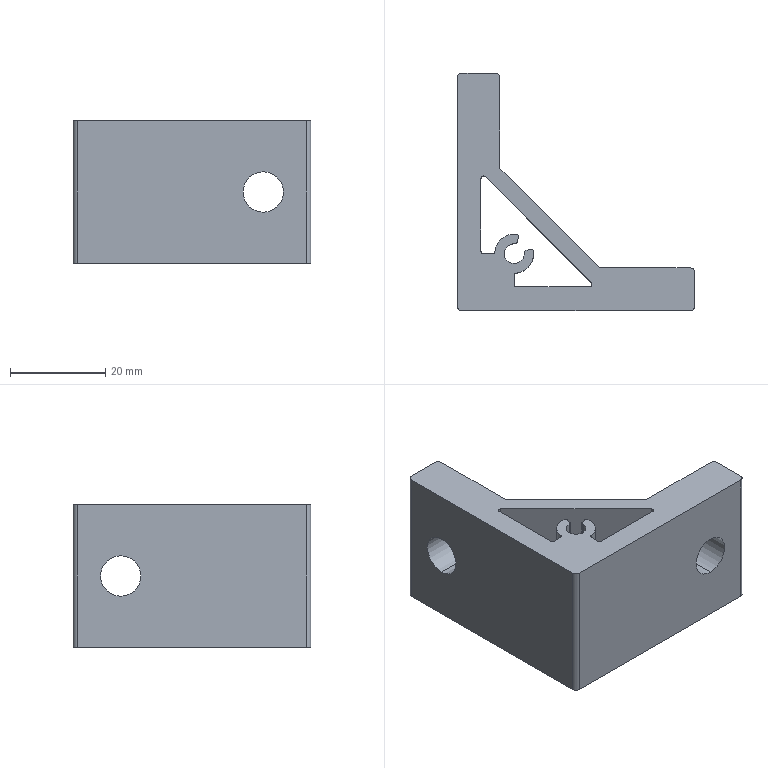Part | SolidWorks | features BaseBody 1 | 1 solid | 41 faces | box 50 x 50 x 30 mm | volume 23521 mm3 | cylinder 25 | plane 16 | commonest cylinder face diameters 1 x11 2 x5 8.5 x4 4.2 x3 8.2 x2
STEP:
#1=CARTESIAN_POINT('',(0.,40.,-10.75));
#2=VERTEX_POINT('',#1);
#3=CARTESIAN_POINT('',(0.,40.,-19.25));
#4=VERTEX_POINT('',#3);
#5=CARTESIAN_POINT('',(0.,40.,-15.));
#6=DIRECTION('',(1.,0.,0.));
#7=DIRECTION('',(0.,0.,-1.));
#8=AXIS2_PLACEMENT_3D('',#5,#6,#7);
#9=CIRCLE('',#8,4.25);
#10=EDGE_CURVE('',#2,#4,#9,.T.);
#11=ORIENTED_EDGE('',*,*,#10,.F.);
#12=CARTESIAN_POINT('',(9.,40.,-10.75));
#13=VERTEX_POINT('',#12);
#14=CARTESIAN_POINT('',(30.,40.,-10.75));
#15=DIRECTION('',(1.,0.,0.));
#16=VECTOR('',#15,1000.);
#17=LINE('',#14,#16);
#18=EDGE_CURVE('',#2,#13,#17,.T.);
#19=ORIENTED_EDGE('',*,*,#18,.T.);
#20=CARTESIAN_POINT('',(9.,40.,-19.25));
#21=VERTEX_POINT('',#20);
#22=CARTESIAN_POINT('',(9.,40.,-15.));
#23=DIRECTION('',(-1.,0.,0.));
#24=DIRECTION('',(0.,0.,-1.));
#25=AXIS2_PLACEMENT_3D('',#22,#23,#24);
#26=CIRCLE('',#25,4.25);
#27=EDGE_CURVE('',#21,#13,#26,.T.);
#28=ORIENTED_EDGE('',*,*,#27,.F.);
#29=CARTESIAN_POINT('',(30.,40.,-19.25));
#30=DIRECTION('',(1.,0.,0.));
#31=VECTOR('',#30,1000.);
#32=LINE('',#29,#31);
#33=EDGE_CURVE('',#4,#21,#32,.T.);
#34=ORIENTED_EDGE('',*,*,#33,.F.);
#35=EDGE_LOOP('',(#11,#19,#28,#34));
#36=FACE_OUTER_BOUND('',#35,.T.);
#37=CARTESIAN_POINT('',(30.,40.,-15.));
#38=DIRECTION('',(1.,0.,0.));
#39=DIRECTION('',(0.,0.,-1.));
#40=AXIS2_PLACEMENT_3D('',#37,#38,#39);
#41=CYLINDRICAL_SURFACE('',#40,4.25);
#42=ADVANCED_FACE('',(#36),#41,.F.);
#43=CARTESIAN_POINT('',(14.1,12.,0.));
#44=VERTEX_POINT('',#43);
#45=CARTESIAN_POINT('',(9.9,12.,0.));
#46=VERTEX_POINT('',#45);
#47=CARTESIAN_POINT('',(12.,12.,0.));
#48=DIRECTION('',(0.,0.,-1.));
#49=DIRECTION('',(-1.,0.,0.));
#50=AXIS2_PLACEMENT_3D('',#47,#48,#49);
#51=CIRCLE('',#50,2.1);
#52=EDGE_CURVE('',#44,#46,#51,.T.);
#53=ORIENTED_EDGE('',*,*,#52,.F.);
#54=CARTESIAN_POINT('',(14.1,12.,-30.));
#55=VERTEX_POINT('',#54);
#56=CARTESIAN_POINT('',(14.1,12.,-30.));
#57=DIRECTION('',(0.,0.,-1.));
#58=VECTOR('',#57,1000.);
#59=LINE('',#56,#58);
#60=EDGE_CURVE('',#44,#55,#59,.T.);
#61=ORIENTED_EDGE('',*,*,#60,.T.);
#62=CARTESIAN_POINT('',(9.9,12.,-30.));
#63=VERTEX_POINT('',#62);
#64=CARTESIAN_POINT('',(12.,12.,-30.));
#65=DIRECTION('',(0.,0.,-1.));
#66=DIRECTION('',(-1.,0.,0.));
#67=AXIS2_PLACEMENT_3D('',#64,#65,#66);
#68=CIRCLE('',#67,2.1);
#69=EDGE_CURVE('',#55,#63,#68,.T.);
#70=ORIENTED_EDGE('',*,*,#69,.T.);
#71=CARTESIAN_POINT('',(9.9,12.,-30.));
#72=DIRECTION('',(0.,0.,-1.));
#73=VECTOR('',#72,1000.);
#74=LINE('',#71,#73);
#75=EDGE_CURVE('',#46,#63,#74,.T.);
#76=ORIENTED_EDGE('',*,*,#75,.F.);
#77=EDGE_LOOP('',(#53,#61,#70,#76));
#78=FACE_OUTER_BOUND('',#77,.T.);
#79=CARTESIAN_POINT('',(12.,12.,-30.));
#80=DIRECTION('',(0.,0.,-1.));
#81=DIRECTION('',(-1.,0.,0.));
#82=AXIS2_PLACEMENT_3D('',#79,#80,#81);
#83=CYLINDRICAL_SURFACE('',#82,2.1);
#84=ADVANCED_FACE('',(#78),#83,.F.);
#85=CARTESIAN_POINT('',(12.143,14.095,0.));
#86=VERTEX_POINT('',#85);
#87=CARTESIAN_POINT('',(12.,12.,0.));
#88=DIRECTION('',(0.,0.,-1.));
#89=DIRECTION('',(-1.,0.,0.));
#90=AXIS2_PLACEMENT_3D('',#87,#88,#89);
#91=CIRCLE('',#90,2.1);
#92=EDGE_CURVE('',#46,#86,#91,.T.);
#93=ORIENTED_EDGE('',*,*,#92,.F.);
#94=ORIENTED_EDGE('',*,*,#75,.T.);
#95=CARTESIAN_POINT('',(12.143,14.095,-30.));
#96=VERTEX_POINT('',#95);
#97=CARTESIAN_POINT('',(12.,12.,-30.));
#98=DIRECTION('',(0.,0.,-1.));
#99=DIRECTION('',(-1.,0.,0.));
#100=AXIS2_PLACEMENT_3D('',#97,#98,#99);
#101=CIRCLE('',#100,2.1);
#102=EDGE_CURVE('',#63,#96,#101,.T.);
#103=ORIENTED_EDGE('',*,*,#102,.T.);
#104=CARTESIAN_POINT('',(12.143,14.095,-30.));
#105=DIRECTION('',(0.,0.,-1.));
#106=VECTOR('',#105,1000.);
#107=LINE('',#104,#106);
#108=EDGE_CURVE('',#86,#96,#107,.T.);
#109=ORIENTED_EDGE('',*,*,#108,.F.);
#110=EDGE_LOOP('',(#93,#94,#103,#109));
#111=FACE_OUTER_BOUND('',#110,.T.);
#112=CARTESIAN_POINT('',(12.,12.,-30.));
#113=DIRECTION('',(0.,0.,-1.));
#114=DIRECTION('',(-1.,0.,0.));
#115=AXIS2_PLACEMENT_3D('',#112,#113,#114);
#116=CYLINDRICAL_SURFACE('',#115,2.1);
#117=ADVANCED_FACE('',(#111),#116,.F.);
#118=CARTESIAN_POINT('',(40.,0.,-19.25));
#119=VERTEX_POINT('',#118);
#120=CARTESIAN_POINT('',(40.,0.,-10.75));
#121=VERTEX_POINT('',#120);
#122=CARTESIAN_POINT('',(40.,0.,-15.));
#123=DIRECTION('',(0.,1.,0.));
#124=DIRECTION('',(0.,0.,1.));
#125=AXIS2_PLACEMENT_3D('',#122,#123,#124);
#126=CIRCLE('',#125,4.25);
#127=EDGE_CURVE('',#119,#121,#126,.T.);
#128=ORIENTED_EDGE('',*,*,#127,.F.);
#129=CARTESIAN_POINT('',(40.,9.,-19.25));
#130=VERTEX_POINT('',#129);
#131=CARTESIAN_POINT('',(40.,30.,-19.25));
#132=DIRECTION('',(0.,1.,0.));
#133=VECTOR('',#132,1000.);
#134=LINE('',#131,#133);
#135=EDGE_CURVE('',#119,#130,#134,.T.);
#136=ORIENTED_EDGE('',*,*,#135,.T.);
#137=CARTESIAN_POINT('',(40.,9.,-10.75));
#138=VERTEX_POINT('',#137);
#139=CARTESIAN_POINT('',(40.,9.,-15.));
#140=DIRECTION('',(0.,-1.,0.));
#141=DIRECTION('',(0.,0.,1.));
#142=AXIS2_PLACEMENT_3D('',#139,#140,#141);
#143=CIRCLE('',#142,4.25);
#144=EDGE_CURVE('',#138,#130,#143,.T.);
#145=ORIENTED_EDGE('',*,*,#144,.F.);
#146=CARTESIAN_POINT('',(40.,30.,-10.75));
#147=DIRECTION('',(0.,1.,0.));
#148=VECTOR('',#147,1000.);
#149=LINE('',#146,#148);
#150=EDGE_CURVE('',#121,#138,#149,.T.);
#151=ORIENTED_EDGE('',*,*,#150,.F.);
#152=EDGE_LOOP('',(#128,#136,#145,#151));
#153=FACE_OUTER_BOUND('',#152,.T.);
#154=CARTESIAN_POINT('',(40.,30.,-15.));
#155=DIRECTION('',(0.,1.,0.));
#156=DIRECTION('',(0.,0.,1.));
#157=AXIS2_PLACEMENT_3D('',#154,#155,#156);
#158=CYLINDRICAL_SURFACE('',#157,4.25);
#159=ADVANCED_FACE('',(#153),#158,.F.);
#160=CARTESIAN_POINT('',(14.095,12.144,0.));
#161=VERTEX_POINT('',#160);
#162=CARTESIAN_POINT('',(14.094,12.178,0.));
#163=VERTEX_POINT('',#162);
#164=CARTESIAN_POINT('',(14.594,12.178,0.));
#165=DIRECTION('',(0.,0.,-1.));
#166=DIRECTION('',(-1.,0.,0.));
#167=AXIS2_PLACEMENT_3D('',#164,#165,#166);
#168=CIRCLE('',#167,0.5);
#169=EDGE_CURVE('',#161,#163,#168,.T.);
#170=ORIENTED_EDGE('',*,*,#169,.T.);
#171=CARTESIAN_POINT('',(14.094,12.178,-30.));
#172=VERTEX_POINT('',#171);
#173=CARTESIAN_POINT('',(14.094,12.178,-30.));
#174=DIRECTION('',(0.,0.,-1.));
#175=VECTOR('',#174,1000.);
#176=LINE('',#173,#175);
#177=EDGE_CURVE('',#163,#172,#176,.T.);
#178=ORIENTED_EDGE('',*,*,#177,.T.);
#179=CARTESIAN_POINT('',(14.095,12.144,-30.));
#180=VERTEX_POINT('',#179);
#181=CARTESIAN_POINT('',(14.594,12.178,-30.));
#182=DIRECTION('',(0.,0.,1.));
#183=DIRECTION('',(-1.,0.,0.));
#184=AXIS2_PLACEMENT_3D('',#181,#182,#183);
#185=CIRCLE('',#184,0.5);
#186=EDGE_CURVE('',#172,#180,#185,.T.);
#187=ORIENTED_EDGE('',*,*,#186,.T.);
#188=CARTESIAN_POINT('',(14.095,12.144,-30.));
#189=DIRECTION('',(0.,0.,1.));
#190=VECTOR('',#189,1000.);
#191=LINE('',#188,#190);
#192=EDGE_CURVE('',#180,#161,#191,.T.);
#193=ORIENTED_EDGE('',*,*,#192,.T.);
#194=EDGE_LOOP('',(#170,#178,#187,#193));
#195=FACE_OUTER_BOUND('',#194,.T.);
#196=CARTESIAN_POINT('',(14.594,12.178,-30.));
#197=DIRECTION('',(0.,0.,-1.));
#198=DIRECTION('',(-1.,0.,0.));
#199=AXIS2_PLACEMENT_3D('',#196,#197,#198);
#200=CYLINDRICAL_SURFACE('',#199,0.5);
#201=ADVANCED_FACE('',(#195),#200,.T.);
#202=CARTESIAN_POINT('',(0.,49.,-30.));
#203=VERTEX_POINT('',#202);
#204=CARTESIAN_POINT('',(0.,1.,-30.));
#205=VERTEX_POINT('',#204);
#206=CARTESIAN_POINT('',(0.,49.,-30.));
#207=DIRECTION('',(0.,-1.,0.));
#208=VECTOR('',#207,1000.);
#209=LINE('',#206,#208);
#210=EDGE_CURVE('',#203,#205,#209,.T.);
#211=ORIENTED_EDGE('',*,*,#210,.T.);
#212=CARTESIAN_POINT('',(0.,1.,0.));
#213=VERTEX_POINT('',#212);
#214=CARTESIAN_POINT('',(0.,1.,-30.));
#215=DIRECTION('',(0.,0.,1.));
#216=VECTOR('',#215,1000.);
#217=LINE('',#214,#216);
#218=EDGE_CURVE('',#205,#213,#217,.T.);
#219=ORIENTED_EDGE('',*,*,#218,.T.);
#220=CARTESIAN_POINT('',(0.,49.,0.));
#221=VERTEX_POINT('',#220);
#222=CARTESIAN_POINT('',(0.,49.,0.));
#223=DIRECTION('',(0.,1.,0.));
#224=VECTOR('',#223,1000.);
#225=LINE('',#222,#224);
#226=EDGE_CURVE('',#213,#221,#225,.T.);
#227=ORIENTED_EDGE('',*,*,#226,.T.);
#228=CARTESIAN_POINT('',(0.,49.,-30.));
#229=DIRECTION('',(0.,0.,-1.));
#230=VECTOR('',#229,1000.);
#231=LINE('',#228,#230);
#232=EDGE_CURVE('',#221,#203,#231,.T.);
#233=ORIENTED_EDGE('',*,*,#232,.T.);
#234=EDGE_LOOP('',(#211,#219,#227,#233));
#235=FACE_OUTER_BOUND('',#234,.T.);
#236=CARTESIAN_POINT('',(0.,40.,-15.));
#237=DIRECTION('',(1.,0.,0.));
#238=DIRECTION('',(0.,0.,-1.));
#239=AXIS2_PLACEMENT_3D('',#236,#237,#238);
#240=CIRCLE('',#239,4.25);
#241=EDGE_CURVE('',#4,#2,#240,.T.);
#242=ORIENTED_EDGE('',*,*,#241,.T.);
#243=ORIENTED_EDGE('',*,*,#10,.T.);
#244=EDGE_LOOP('',(#242,#243));
#245=FACE_BOUND('',#244,.T.);
#246=CARTESIAN_POINT('',(0.,49.,-30.));
#247=DIRECTION('',(-1.,0.,0.));
#248=DIRECTION('',(0.,0.,1.));
#249=AXIS2_PLACEMENT_3D('',#246,#247,#248);
#250=PLANE('',#249);
#251=ADVANCED_FACE('',(#235,#245),#250,.T.);
#252=CARTESIAN_POINT('',(1.,0.,-30.));
#253=VERTEX_POINT('',#252);
#254=CARTESIAN_POINT('',(1.,1.,-30.));
#255=DIRECTION('',(0.,0.,1.));
#256=DIRECTION('',(-1.,0.,0.));
#257=AXIS2_PLACEMENT_3D('',#254,#255,#256);
#258=CIRCLE('',#257,1.);
#259=EDGE_CURVE('',#205,#253,#258,.T.);
#260=ORIENTED_EDGE('',*,*,#259,.T.);
#261=CARTESIAN_POINT('',(1.,0.,0.));
#262=VERTEX_POINT('',#261);
#263=CARTESIAN_POINT('',(1.,0.,-30.));
#264=DIRECTION('',(0.,0.,1.));
#265=VECTOR('',#264,1000.);
#266=LINE('',#263,#265);
#267=EDGE_CURVE('',#253,#262,#266,.T.);
#268=ORIENTED_EDGE('',*,*,#267,.T.);
#269=CARTESIAN_POINT('',(1.,1.,0.));
#270=DIRECTION('',(0.,0.,-1.));
#271=DIRECTION('',(-1.,0.,0.));
#272=AXIS2_PLACEMENT_3D('',#269,#270,#271);
#273=CIRCLE('',#272,1.);
#274=EDGE_CURVE('',#262,#213,#273,.T.);
#275=ORIENTED_EDGE('',*,*,#274,.T.);
#276=ORIENTED_EDGE('',*,*,#218,.F.);
#277=EDGE_LOOP('',(#260,#268,#275,#276));
#278=FACE_OUTER_BOUND('',#277,.T.);
#279=CARTESIAN_POINT('',(1.,1.,-30.));
#280=DIRECTION('',(0.,0.,-1.));
#281=DIRECTION('',(-1.,0.,0.));
#282=AXIS2_PLACEMENT_3D('',#279,#280,#281);
#283=CYLINDRICAL_SURFACE('',#282,1.);
#284=ADVANCED_FACE('',(#278),#283,.T.);
#285=CARTESIAN_POINT('',(8.,50.,-30.));
#286=VERTEX_POINT('',#285);
#287=CARTESIAN_POINT('',(1.,50.,-30.));
#288=VERTEX_POINT('',#287);
#289=CARTESIAN_POINT('',(1.,50.,-30.));
#290=DIRECTION('',(-1.,0.,0.));
#291=VECTOR('',#290,1000.);
#292=LINE('',#289,#291);
#293=EDGE_CURVE('',#286,#288,#292,.T.);
#294=ORIENTED_EDGE('',*,*,#293,.F.);
#295=CARTESIAN_POINT('',(9.,49.,-30.));
#296=VERTEX_POINT('',#295);
#297=CARTESIAN_POINT('',(8.,49.,-30.));
#298=DIRECTION('',(0.,0.,1.));
#299=DIRECTION('',(-1.,0.,0.));
#300=AXIS2_PLACEMENT_3D('',#297,#298,#299);
#301=CIRCLE('',#300,1.);
#302=EDGE_CURVE('',#296,#286,#301,.T.);
#303=ORIENTED_EDGE('',*,*,#302,.F.);
#304=CARTESIAN_POINT('',(9.,30.,-30.));
#305=VERTEX_POINT('',#304);
#306=CARTESIAN_POINT('',(9.,49.,-30.));
#307=DIRECTION('',(0.,1.,0.));
#308=VECTOR('',#307,1000.);
#309=LINE('',#306,#308);
#310=EDGE_CURVE('',#305,#296,#309,.T.);
#311=ORIENTED_EDGE('',*,*,#310,.F.);
#312=CARTESIAN_POINT('',(30.,9.,-30.));
#313=VERTEX_POINT('',#312);
#314=CARTESIAN_POINT('',(30.,9.,-30.));
#315=DIRECTION('',(-0.7071,0.7071,0.));
#316=VECTOR('',#315,1000.);
#317=LINE('',#314,#316);
#318=EDGE_CURVE('',#313,#305,#317,.T.);
#319=ORIENTED_EDGE('',*,*,#318,.F.);
#320=CARTESIAN_POINT('',(49.,9.,-30.));
#321=VERTEX_POINT('',#320);
#322=CARTESIAN_POINT('',(1.,9.,-30.));
#323=DIRECTION('',(-1.,0.,0.));
#324=VECTOR('',#323,1000.);
#325=LINE('',#322,#324);
#326=EDGE_CURVE('',#321,#313,#325,.T.);
#327=ORIENTED_EDGE('',*,*,#326,.F.);
#328=CARTESIAN_POINT('',(50.,8.,-30.));
#329=VERTEX_POINT('',#328);
#330=CARTESIAN_POINT('',(49.,8.,-30.));
#331=DIRECTION('',(0.,0.,1.));
#332=DIRECTION('',(-1.,0.,0.));
#333=AXIS2_PLACEMENT_3D('',#330,#331,#332);
#334=CIRCLE('',#333,1.);
#335=EDGE_CURVE('',#329,#321,#334,.T.);
#336=ORIENTED_EDGE('',*,*,#335,.F.);
#337=CARTESIAN_POINT('',(50.,1.,-30.));
#338=VERTEX_POINT('',#337);
#339=CARTESIAN_POINT('',(50.,49.,-30.));
#340=DIRECTION('',(0.,1.,0.));
#341=VECTOR('',#340,1000.);
#342=LINE('',#339,#341);
#343=EDGE_CURVE('',#338,#329,#342,.T.);
#344=ORIENTED_EDGE('',*,*,#343,.F.);
#345=CARTESIAN_POINT('',(49.,0.,-30.));
#346=VERTEX_POINT('',#345);
#347=CARTESIAN_POINT('',(49.,1.,-30.));
#348=DIRECTION('',(0.,0.,1.));
#349=DIRECTION('',(-1.,0.,0.));
#350=AXIS2_PLACEMENT_3D('',#347,#348,#349);
#351=CIRCLE('',#350,1.);
#352=EDGE_CURVE('',#346,#338,#351,.T.);
#353=ORIENTED_EDGE('',*,*,#352,.F.);
#354=CARTESIAN_POINT('',(1.,0.,-30.));
#355=DIRECTION('',(1.,0.,0.));
#356=VECTOR('',#355,1000.);
#357=LINE('',#354,#356);
#358=EDGE_CURVE('',#253,#346,#357,.T.);
#359=ORIENTED_EDGE('',*,*,#358,.F.);
#360=ORIENTED_EDGE('',*,*,#259,.F.);
#361=ORIENTED_EDGE('',*,*,#210,.F.);
#362=CARTESIAN_POINT('',(1.,49.,-30.));
#363=DIRECTION('',(0.,0.,1.));
#364=DIRECTION('',(-1.,0.,0.));
#365=AXIS2_PLACEMENT_3D('',#362,#363,#364);
#366=CIRCLE('',#365,1.);
#367=EDGE_CURVE('',#288,#203,#366,.T.);
#368=ORIENTED_EDGE('',*,*,#367,.F.);
#369=EDGE_LOOP('',(#294,#303,#311,#319,#327,#336,#344,#353,#359,#360,#361,#368));
#370=FACE_OUTER_BOUND('',#369,.T.);
#371=CARTESIAN_POINT('',(5.,12.5,-30.));
#372=VERTEX_POINT('',#371);
#373=CARTESIAN_POINT('',(5.5,12.,-30.));
#374=VERTEX_POINT('',#373);
#375=CARTESIAN_POINT('',(5.5,12.5,-30.));
#376=DIRECTION('',(0.,0.,1.));
#377=DIRECTION('',(-1.,0.,0.));
#378=AXIS2_PLACEMENT_3D('',#375,#376,#377);
#379=CIRCLE('',#378,0.5);
#380=EDGE_CURVE('',#372,#374,#379,.T.);
#381=ORIENTED_EDGE('',*,*,#380,.T.);
#382=CARTESIAN_POINT('',(7.427,12.,-30.));
#383=VERTEX_POINT('',#382);
#384=CARTESIAN_POINT('',(1.,12.,-30.));
#385=DIRECTION('',(-1.,0.,0.));
#386=VECTOR('',#385,1000.);
#387=LINE('',#384,#386);
#388=EDGE_CURVE('',#383,#374,#387,.T.);
#389=ORIENTED_EDGE('',*,*,#388,.F.);
#390=CARTESIAN_POINT('',(7.924,12.446,-30.));
#391=VERTEX_POINT('',#390);
#392=CARTESIAN_POINT('',(7.427,12.5,-30.));
#393=DIRECTION('',(0.,0.,1.));
#394=DIRECTION('',(-1.,0.,0.));
#395=AXIS2_PLACEMENT_3D('',#392,#393,#394);
#396=CIRCLE('',#395,0.5);
#397=EDGE_CURVE('',#383,#391,#396,.T.);
#398=ORIENTED_EDGE('',*,*,#397,.T.);
#399=CARTESIAN_POINT('',(12.501,16.07,-30.));
#400=VERTEX_POINT('',#399);
#401=CARTESIAN_POINT('',(12.,12.001,-30.));
#402=DIRECTION('',(0.,0.,1.));
#403=DIRECTION('',(-1.,0.,0.));
#404=AXIS2_PLACEMENT_3D('',#401,#402,#403);
#405=CIRCLE('',#404,4.1);
#406=EDGE_CURVE('',#400,#391,#405,.T.);
#407=ORIENTED_EDGE('',*,*,#406,.F.);
#408=CARTESIAN_POINT('',(12.923,15.444,-30.));
#409=VERTEX_POINT('',#408);
#410=CARTESIAN_POINT('',(12.44,15.574,-30.));
#411=DIRECTION('',(0.,0.,1.));
#412=DIRECTION('',(-1.,0.,0.));
#413=AXIS2_PLACEMENT_3D('',#410,#411,#412);
#414=CIRCLE('',#413,0.5);
#415=EDGE_CURVE('',#409,#400,#414,.T.);
#416=ORIENTED_EDGE('',*,*,#415,.F.);
#417=CARTESIAN_POINT('',(12.66,14.464,-30.));
#418=VERTEX_POINT('',#417);
#419=CARTESIAN_POINT('',(12.923,15.444,-30.));
#420=DIRECTION('',(-0.2594,-0.9658,0.));
#421=VECTOR('',#420,1000.);
#422=LINE('',#419,#421);
#423=EDGE_CURVE('',#409,#418,#422,.T.);
#424=ORIENTED_EDGE('',*,*,#423,.T.);
#425=CARTESIAN_POINT('',(12.177,14.594,-30.));
#426=DIRECTION('',(0.,0.,1.));
#427=DIRECTION('',(-1.,0.,0.));
#428=AXIS2_PLACEMENT_3D('',#425,#426,#427);
#429=CIRCLE('',#428,0.5);
#430=EDGE_CURVE('',#96,#418,#429,.T.);
#431=ORIENTED_EDGE('',*,*,#430,.F.);
#432=ORIENTED_EDGE('',*,*,#102,.F.);
#433=ORIENTED_EDGE('',*,*,#69,.F.);
#434=CARTESIAN_POINT('',(12.,12.,-30.));
#435=DIRECTION('',(0.,0.,-1.));
#436=DIRECTION('',(-1.,0.,0.));
#437=AXIS2_PLACEMENT_3D('',#434,#435,#436);
#438=CIRCLE('',#437,2.1);
#439=EDGE_CURVE('',#180,#55,#438,.T.);
#440=ORIENTED_EDGE('',*,*,#439,.F.);
#441=ORIENTED_EDGE('',*,*,#186,.F.);
#442=CARTESIAN_POINT('',(14.465,12.661,-30.));
#443=VERTEX_POINT('',#442);
#444=CARTESIAN_POINT('',(14.594,12.178,-30.));
#445=DIRECTION('',(0.,0.,1.));
#446=DIRECTION('',(-1.,0.,0.));
#447=AXIS2_PLACEMENT_3D('',#444,#445,#446);
#448=CIRCLE('',#447,0.5);
#449=EDGE_CURVE('',#443,#172,#448,.T.);
#450=ORIENTED_EDGE('',*,*,#449,.F.);
#451=CARTESIAN_POINT('',(15.444,12.923,-30.));
#452=VERTEX_POINT('',#451);
#453=CARTESIAN_POINT('',(14.465,12.661,-30.));
#454=DIRECTION('',(0.9661,0.2583,0.));
#455=VECTOR('',#454,1000.);
#456=LINE('',#453,#455);
#457=EDGE_CURVE('',#443,#452,#456,.T.);
#458=ORIENTED_EDGE('',*,*,#457,.T.);
#459=CARTESIAN_POINT('',(16.069,12.501,-30.));
#460=VERTEX_POINT('',#459);
#461=CARTESIAN_POINT('',(15.573,12.44,-30.));
#462=DIRECTION('',(0.,0.,1.));
#463=DIRECTION('',(-1.,0.,0.));
#464=AXIS2_PLACEMENT_3D('',#461,#462,#463);
#465=CIRCLE('',#464,0.5);
#466=EDGE_CURVE('',#460,#452,#465,.T.);
#467=ORIENTED_EDGE('',*,*,#466,.F.);
#468=CARTESIAN_POINT('',(12.446,7.925,-30.));
#469=VERTEX_POINT('',#468);
#470=CARTESIAN_POINT('',(12.,12.001,-30.));
#471=DIRECTION('',(0.,0.,1.));
#472=DIRECTION('',(-1.,0.,0.));
#473=AXIS2_PLACEMENT_3D('',#470,#471,#472);
#474=CIRCLE('',#473,4.1);
#475=EDGE_CURVE('',#469,#460,#474,.T.);
#476=ORIENTED_EDGE('',*,*,#475,.F.);
#477=CARTESIAN_POINT('',(12.,7.428,-30.));
#478=VERTEX_POINT('',#477);
#479=CARTESIAN_POINT('',(12.5,7.428,-30.));
#480=DIRECTION('',(0.,0.,1.));
#481=DIRECTION('',(-1.,0.,0.));
#482=AXIS2_PLACEMENT_3D('',#479,#480,#481);
#483=CIRCLE('',#482,0.5);
#484=EDGE_CURVE('',#469,#478,#483,.T.);
#485=ORIENTED_EDGE('',*,*,#484,.T.);
#486=CARTESIAN_POINT('',(12.,5.5,-30.));
#487=VERTEX_POINT('',#486);
#488=CARTESIAN_POINT('',(12.,49.,-30.));
#489=DIRECTION('',(0.,1.,0.));
#490=VECTOR('',#489,1000.);
#491=LINE('',#488,#490);
#492=EDGE_CURVE('',#487,#478,#491,.T.);
#493=ORIENTED_EDGE('',*,*,#492,.F.);
#494=CARTESIAN_POINT('',(12.5,5.,-30.));
#495=VERTEX_POINT('',#494);
#496=CARTESIAN_POINT('',(12.5,5.5,-30.));
#497=DIRECTION('',(0.,0.,1.));
#498=DIRECTION('',(-1.,0.,0.));
#499=AXIS2_PLACEMENT_3D('',#496,#497,#498);
#500=CIRCLE('',#499,0.5);
#501=EDGE_CURVE('',#487,#495,#500,.T.);
#502=ORIENTED_EDGE('',*,*,#501,.T.);
#503=CARTESIAN_POINT('',(27.844,5.,-30.));
#504=VERTEX_POINT('',#503);
#505=CARTESIAN_POINT('',(1.,5.,-30.));
#506=DIRECTION('',(-1.,0.,0.));
#507=VECTOR('',#506,1000.);
#508=LINE('',#505,#507);
#509=EDGE_CURVE('',#504,#495,#508,.T.);
#510=ORIENTED_EDGE('',*,*,#509,.F.);
#511=CARTESIAN_POINT('',(28.197,5.854,-30.));
#512=VERTEX_POINT('',#511);
#513=CARTESIAN_POINT('',(27.844,5.5,-30.));
#514=DIRECTION('',(0.,0.,1.));
#515=DIRECTION('',(-1.,0.,0.));
#516=AXIS2_PLACEMENT_3D('',#513,#514,#515);
#517=CIRCLE('',#516,0.5);
#518=EDGE_CURVE('',#504,#512,#517,.T.);
#519=ORIENTED_EDGE('',*,*,#518,.T.);
#520=CARTESIAN_POINT('',(5.854,28.196,-30.));
#521=VERTEX_POINT('',#520);
#522=CARTESIAN_POINT('',(5.854,28.196,-30.));
#523=DIRECTION('',(0.7071,-0.7071,0.));
#524=VECTOR('',#523,1000.);
#525=LINE('',#522,#524);
#526=EDGE_CURVE('',#521,#512,#525,.T.);
#527=ORIENTED_EDGE('',*,*,#526,.F.);
#528=CARTESIAN_POINT('',(5.,27.843,-30.));
#529=VERTEX_POINT('',#528);
#530=CARTESIAN_POINT('',(5.5,27.843,-30.));
#531=DIRECTION('',(0.,0.,1.));
#532=DIRECTION('',(-1.,0.,0.));
#533=AXIS2_PLACEMENT_3D('',#530,#531,#532);
#534=CIRCLE('',#533,0.5);
#535=EDGE_CURVE('',#521,#529,#534,.T.);
#536=ORIENTED_EDGE('',*,*,#535,.T.);
#537=CARTESIAN_POINT('',(5.,49.,-30.));
#538=DIRECTION('',(0.,1.,0.));
#539=VECTOR('',#538,1000.);
#540=LINE('',#537,#539);
#541=EDGE_CURVE('',#372,#529,#540,.T.);
#542=ORIENTED_EDGE('',*,*,#541,.F.);
#543=EDGE_LOOP('',(#381,#389,#398,#407,#416,#424,#431,#432,#433,#440,#441,#450,#458,#467,#476,#485,#493,#502,#510,#519,#527,#536,#542));
#544=FACE_BOUND('',#543,.T.);
#545=CARTESIAN_POINT('',(1.,49.,-30.));
#546=DIRECTION('',(0.,0.,1.));
#547=DIRECTION('',(1.,0.,0.));
#548=AXIS2_PLACEMENT_3D('',#545,#546,#547);
#549=PLANE('',#548);
#550=ADVANCED_FACE('',(#370,#544),#549,.F.);
#551=ORIENTED_EDGE('',*,*,#367,.T.);
#552=ORIENTED_EDGE('',*,*,#232,.F.);
#553=CARTESIAN_POINT('',(1.,50.,0.));
#554=VERTEX_POINT('',#553);
#555=CARTESIAN_POINT('',(1.,49.,0.));
#556=DIRECTION('',(0.,0.,-1.));
#557=DIRECTION('',(-1.,0.,0.));
#558=AXIS2_PLACEMENT_3D('',#555,#556,#557);
#559=CIRCLE('',#558,1.);
#560=EDGE_CURVE('',#221,#554,#559,.T.);
#561=ORIENTED_EDGE('',*,*,#560,.T.);
#562=CARTESIAN_POINT('',(1.,50.,-30.));
#563=DIRECTION('',(0.,0.,-1.));
#564=VECTOR('',#563,1000.);
#565=LINE('',#562,#564);
#566=EDGE_CURVE('',#554,#288,#565,.T.);
#567=ORIENTED_EDGE('',*,*,#566,.T.);
#568=EDGE_LOOP('',(#551,#552,#561,#567));
#569=FACE_OUTER_BOUND('',#568,.T.);
#570=CARTESIAN_POINT('',(1.,49.,-30.));
#571=DIRECTION('',(0.,0.,-1.));
#572=DIRECTION('',(-1.,0.,0.));
#573=AXIS2_PLACEMENT_3D('',#570,#571,#572);
#574=CYLINDRICAL_SURFACE('',#573,1.);
#575=ADVANCED_FACE('',(#569),#574,.T.);
#576=CARTESIAN_POINT('',(8.,50.,0.));
#577=VERTEX_POINT('',#576);
#578=CARTESIAN_POINT('',(9.,49.,0.));
#579=VERTEX_POINT('',#578);
#580=CARTESIAN_POINT('',(8.,49.,0.));
#581=DIRECTION('',(0.,0.,-1.));
#582=DIRECTION('',(-1.,0.,0.));
#583=AXIS2_PLACEMENT_3D('',#580,#581,#582);
#584=CIRCLE('',#583,1.);
#585=EDGE_CURVE('',#577,#579,#584,.T.);
#586=ORIENTED_EDGE('',*,*,#585,.F.);
#587=CARTESIAN_POINT('',(1.,50.,0.));
#588=DIRECTION('',(-1.,0.,0.));
#589=VECTOR('',#588,1000.);
#590=LINE('',#587,#589);
#591=EDGE_CURVE('',#577,#554,#590,.T.);
#592=ORIENTED_EDGE('',*,*,#591,.T.);
#593=ORIENTED_EDGE('',*,*,#560,.F.);
#594=ORIENTED_EDGE('',*,*,#226,.F.);
#595=ORIENTED_EDGE('',*,*,#274,.F.);
#596=CARTESIAN_POINT('',(49.,0.,0.));
#597=VERTEX_POINT('',#596);
#598=CARTESIAN_POINT('',(1.,0.,0.));
#599=DIRECTION('',(1.,0.,0.));
#600=VECTOR('',#599,1000.);
#601=LINE('',#598,#600);
#602=EDGE_CURVE('',#262,#597,#601,.T.);
#603=ORIENTED_EDGE('',*,*,#602,.T.);
#604=CARTESIAN_POINT('',(50.,1.,0.));
#605=VERTEX_POINT('',#604);
#606=CARTESIAN_POINT('',(49.,1.,0.));
#607=DIRECTION('',(0.,0.,-1.));
#608=DIRECTION('',(-1.,0.,0.));
#609=AXIS2_PLACEMENT_3D('',#606,#607,#608);
#610=CIRCLE('',#609,1.);
#611=EDGE_CURVE('',#605,#597,#610,.T.);
#612=ORIENTED_EDGE('',*,*,#611,.F.);
#613=CARTESIAN_POINT('',(50.,8.,0.));
#614=VERTEX_POINT('',#613);
#615=CARTESIAN_POINT('',(50.,49.,0.));
#616=DIRECTION('',(0.,1.,0.));
#617=VECTOR('',#616,1000.);
#618=LINE('',#615,#617);
#619=EDGE_CURVE('',#605,#614,#618,.T.);
#620=ORIENTED_EDGE('',*,*,#619,.T.);
#621=CARTESIAN_POINT('',(49.,9.,0.));
#622=VERTEX_POINT('',#621);
#623=CARTESIAN_POINT('',(49.,8.,0.));
#624=DIRECTION('',(0.,0.,-1.));
#625=DIRECTION('',(-1.,0.,0.));
#626=AXIS2_PLACEMENT_3D('',#623,#624,#625);
#627=CIRCLE('',#626,1.);
#628=EDGE_CURVE('',#622,#614,#627,.T.);
#629=ORIENTED_EDGE('',*,*,#628,.F.);
#630=CARTESIAN_POINT('',(30.,9.,0.));
#631=VERTEX_POINT('',#630);
#632=CARTESIAN_POINT('',(1.,9.,0.));
#633=DIRECTION('',(-1.,0.,0.));
#634=VECTOR('',#633,1000.);
#635=LINE('',#632,#634);
#636=EDGE_CURVE('',#622,#631,#635,.T.);
#637=ORIENTED_EDGE('',*,*,#636,.T.);
#638=CARTESIAN_POINT('',(9.,30.,0.));
#639=VERTEX_POINT('',#638);
#640=CARTESIAN_POINT('',(30.,9.,0.));
#641=DIRECTION('',(-0.7071,0.7071,0.));
#642=VECTOR('',#641,1000.);
#643=LINE('',#640,#642);
#644=EDGE_CURVE('',#631,#639,#643,.T.);
#645=ORIENTED_EDGE('',*,*,#644,.T.);
#646=CARTESIAN_POINT('',(9.,49.,0.));
#647=DIRECTION('',(0.,1.,0.));
#648=VECTOR('',#647,1000.);
#649=LINE('',#646,#648);
#650=EDGE_CURVE('',#639,#579,#649,.T.);
#651=ORIENTED_EDGE('',*,*,#650,.T.);
#652=EDGE_LOOP('',(#586,#592,#593,#594,#595,#603,#612,#620,#629,#637,#645,#651));
#653=FACE_OUTER_BOUND('',#652,.T.);
#654=CARTESIAN_POINT('',(7.427,12.,0.));
#655=VERTEX_POINT('',#654);
#656=CARTESIAN_POINT('',(5.5,12.,0.));
#657=VERTEX_POINT('',#656);
#658=CARTESIAN_POINT('',(1.,12.,0.));
#659=DIRECTION('',(-1.,0.,0.));
#660=VECTOR('',#659,1000.);
#661=LINE('',#658,#660);
#662=EDGE_CURVE('',#655,#657,#661,.T.);
#663=ORIENTED_EDGE('',*,*,#662,.T.);
#664=CARTESIAN_POINT('',(5.,12.5,0.));
#665=VERTEX_POINT('',#664);
#666=CARTESIAN_POINT('',(5.5,12.5,0.));
#667=DIRECTION('',(0.,0.,-1.));
#668=DIRECTION('',(-1.,0.,0.));
#669=AXIS2_PLACEMENT_3D('',#666,#667,#668);
#670=CIRCLE('',#669,0.5);
#671=EDGE_CURVE('',#657,#665,#670,.T.);
#672=ORIENTED_EDGE('',*,*,#671,.T.);
#673=CARTESIAN_POINT('',(5.,27.843,0.));
#674=VERTEX_POINT('',#673);
#675=CARTESIAN_POINT('',(5.,49.,0.));
#676=DIRECTION('',(0.,1.,0.));
#677=VECTOR('',#676,1000.);
#678=LINE('',#675,#677);
#679=EDGE_CURVE('',#665,#674,#678,.T.);
#680=ORIENTED_EDGE('',*,*,#679,.T.);
#681=CARTESIAN_POINT('',(5.854,28.196,0.));
#682=VERTEX_POINT('',#681);
#683=CARTESIAN_POINT('',(5.5,27.843,0.));
#684=DIRECTION('',(0.,0.,-1.));
#685=DIRECTION('',(-1.,0.,0.));
#686=AXIS2_PLACEMENT_3D('',#683,#684,#685);
#687=CIRCLE('',#686,0.5);
#688=EDGE_CURVE('',#674,#682,#687,.T.);
#689=ORIENTED_EDGE('',*,*,#688,.T.);
#690=CARTESIAN_POINT('',(28.197,5.854,0.));
#691=VERTEX_POINT('',#690);
#692=CARTESIAN_POINT('',(5.854,28.196,0.));
#693=DIRECTION('',(0.7071,-0.7071,0.));
#694=VECTOR('',#693,1000.);
#695=LINE('',#692,#694);
#696=EDGE_CURVE('',#682,#691,#695,.T.);
#697=ORIENTED_EDGE('',*,*,#696,.T.);
#698=CARTESIAN_POINT('',(27.844,5.,0.));
#699=VERTEX_POINT('',#698);
#700=CARTESIAN_POINT('',(27.844,5.5,0.));
#701=DIRECTION('',(0.,0.,-1.));
#702=DIRECTION('',(-1.,0.,0.));
#703=AXIS2_PLACEMENT_3D('',#700,#701,#702);
#704=CIRCLE('',#703,0.5);
#705=EDGE_CURVE('',#691,#699,#704,.T.);
#706=ORIENTED_EDGE('',*,*,#705,.T.);
#707=CARTESIAN_POINT('',(12.5,5.,0.));
#708=VERTEX_POINT('',#707);
#709=CARTESIAN_POINT('',(1.,5.,0.));
#710=DIRECTION('',(-1.,0.,0.));
#711=VECTOR('',#710,1000.);
#712=LINE('',#709,#711);
#713=EDGE_CURVE('',#699,#708,#712,.T.);
#714=ORIENTED_EDGE('',*,*,#713,.T.);
#715=CARTESIAN_POINT('',(12.,5.5,0.));
#716=VERTEX_POINT('',#715);
#717=CARTESIAN_POINT('',(12.5,5.5,0.));
#718=DIRECTION('',(0.,0.,-1.));
#719=DIRECTION('',(-1.,0.,0.));
#720=AXIS2_PLACEMENT_3D('',#717,#718,#719);
#721=CIRCLE('',#720,0.5);
#722=EDGE_CURVE('',#708,#716,#721,.T.);
#723=ORIENTED_EDGE('',*,*,#722,.T.);
#724=CARTESIAN_POINT('',(12.,7.428,0.));
#725=VERTEX_POINT('',#724);
#726=CARTESIAN_POINT('',(12.,49.,0.));
#727=DIRECTION('',(0.,1.,0.));
#728=VECTOR('',#727,1000.);
#729=LINE('',#726,#728);
#730=EDGE_CURVE('',#716,#725,#729,.T.);
#731=ORIENTED_EDGE('',*,*,#730,.T.);
#732=CARTESIAN_POINT('',(12.446,7.925,0.));
#733=VERTEX_POINT('',#732);
#734=CARTESIAN_POINT('',(12.5,7.428,0.));
#735=DIRECTION('',(0.,0.,-1.));
#736=DIRECTION('',(-1.,0.,0.));
#737=AXIS2_PLACEMENT_3D('',#734,#735,#736);
#738=CIRCLE('',#737,0.5);
#739=EDGE_CURVE('',#725,#733,#738,.T.);
#740=ORIENTED_EDGE('',*,*,#739,.T.);
#741=CARTESIAN_POINT('',(16.069,12.501,0.));
#742=VERTEX_POINT('',#741);
#743=CARTESIAN_POINT('',(12.,12.001,0.));
#744=DIRECTION('',(0.,0.,1.));
#745=DIRECTION('',(-1.,0.,0.));
#746=AXIS2_PLACEMENT_3D('',#743,#744,#745);
#747=CIRCLE('',#746,4.1);
#748=EDGE_CURVE('',#733,#742,#747,.T.);
#749=ORIENTED_EDGE('',*,*,#748,.T.);
#750=CARTESIAN_POINT('',(15.444,12.923,0.));
#751=VERTEX_POINT('',#750);
#752=CARTESIAN_POINT('',(15.573,12.44,0.));
#753=DIRECTION('',(0.,0.,-1.));
#754=DIRECTION('',(-1.,0.,0.));
#755=AXIS2_PLACEMENT_3D('',#752,#753,#754);
#756=CIRCLE('',#755,0.5);
#757=EDGE_CURVE('',#751,#742,#756,.T.);
#758=ORIENTED_EDGE('',*,*,#757,.F.);
#759=CARTESIAN_POINT('',(14.465,12.661,0.));
#760=VERTEX_POINT('',#759);
#761=CARTESIAN_POINT('',(14.465,12.661,0.));
#762=DIRECTION('',(-0.9661,-0.2583,0.));
#763=VECTOR('',#762,1000.);
#764=LINE('',#761,#763);
#765=EDGE_CURVE('',#751,#760,#764,.T.);
#766=ORIENTED_EDGE('',*,*,#765,.T.);
#767=CARTESIAN_POINT('',(14.594,12.178,0.));
#768=DIRECTION('',(0.,0.,-1.));
#769=DIRECTION('',(-1.,0.,0.));
#770=AXIS2_PLACEMENT_3D('',#767,#768,#769);
#771=CIRCLE('',#770,0.5);
#772=EDGE_CURVE('',#163,#760,#771,.T.);
#773=ORIENTED_EDGE('',*,*,#772,.F.);
#774=ORIENTED_EDGE('',*,*,#169,.F.);
#775=CARTESIAN_POINT('',(12.,12.,0.));
#776=DIRECTION('',(0.,0.,-1.));
#777=DIRECTION('',(-1.,0.,0.));
#778=AXIS2_PLACEMENT_3D('',#775,#776,#777);
#779=CIRCLE('',#778,2.1);
#780=EDGE_CURVE('',#161,#44,#779,.T.);
#781=ORIENTED_EDGE('',*,*,#780,.T.);
#782=ORIENTED_EDGE('',*,*,#52,.T.);
#783=ORIENTED_EDGE('',*,*,#92,.T.);
#784=CARTESIAN_POINT('',(12.66,14.464,0.));
#785=VERTEX_POINT('',#784);
#786=CARTESIAN_POINT('',(12.177,14.594,0.));
#787=DIRECTION('',(0.,0.,-1.));
#788=DIRECTION('',(-1.,0.,0.));
#789=AXIS2_PLACEMENT_3D('',#786,#787,#788);
#790=CIRCLE('',#789,0.5);
#791=EDGE_CURVE('',#785,#86,#790,.T.);
#792=ORIENTED_EDGE('',*,*,#791,.F.);
#793=CARTESIAN_POINT('',(12.923,15.444,0.));
#794=VERTEX_POINT('',#793);
#795=CARTESIAN_POINT('',(12.923,15.444,0.));
#796=DIRECTION('',(0.2594,0.9658,0.));
#797=VECTOR('',#796,1000.);
#798=LINE('',#795,#797);
#799=EDGE_CURVE('',#785,#794,#798,.T.);
#800=ORIENTED_EDGE('',*,*,#799,.T.);
#801=CARTESIAN_POINT('',(12.501,16.07,0.));
#802=VERTEX_POINT('',#801);
#803=CARTESIAN_POINT('',(12.44,15.574,0.));
#804=DIRECTION('',(0.,0.,-1.));
#805=DIRECTION('',(-1.,0.,0.));
#806=AXIS2_PLACEMENT_3D('',#803,#804,#805);
#807=CIRCLE('',#806,0.5);
#808=EDGE_CURVE('',#802,#794,#807,.T.);
#809=ORIENTED_EDGE('',*,*,#808,.F.);
#810=CARTESIAN_POINT('',(7.924,12.446,0.));
#811=VERTEX_POINT('',#810);
#812=CARTESIAN_POINT('',(12.,12.001,0.));
#813=DIRECTION('',(0.,0.,1.));
#814=DIRECTION('',(-1.,0.,0.));
#815=AXIS2_PLACEMENT_3D('',#812,#813,#814);
#816=CIRCLE('',#815,4.1);
#817=EDGE_CURVE('',#802,#811,#816,.T.);
#818=ORIENTED_EDGE('',*,*,#817,.T.);
#819=CARTESIAN_POINT('',(7.427,12.5,0.));
#820=DIRECTION('',(0.,0.,-1.));
#821=DIRECTION('',(-1.,0.,0.));
#822=AXIS2_PLACEMENT_3D('',#819,#820,#821);
#823=CIRCLE('',#822,0.5);
#824=EDGE_CURVE('',#811,#655,#823,.T.);
#825=ORIENTED_EDGE('',*,*,#824,.T.);
#826=EDGE_LOOP('',(#663,#672,#680,#689,#697,#706,#714,#723,#731,#740,#749,#758,#766,#773,#774,#781,#782,#783,#792,#800,#809,#818,#825));
#827=FACE_BOUND('',#826,.T.);
#828=CARTESIAN_POINT('',(1.,49.,0.));
#829=DIRECTION('',(0.,0.,1.));
#830=DIRECTION('',(1.,0.,0.));
#831=AXIS2_PLACEMENT_3D('',#828,#829,#830);
#832=PLANE('',#831);
#833=ADVANCED_FACE('',(#653,#827),#832,.T.);
#834=ORIENTED_EDGE('',*,*,#18,.F.);
#835=ORIENTED_EDGE('',*,*,#241,.F.);
#836=ORIENTED_EDGE('',*,*,#33,.T.);
#837=CARTESIAN_POINT('',(9.,40.,-15.));
#838=DIRECTION('',(-1.,0.,0.));
#839=DIRECTION('',(0.,0.,-1.));
#840=AXIS2_PLACEMENT_3D('',#837,#838,#839);
#841=CIRCLE('',#840,4.25);
#842=EDGE_CURVE('',#13,#21,#841,.T.);
#843=ORIENTED_EDGE('',*,*,#842,.F.);
#844=EDGE_LOOP('',(#834,#835,#836,#843));
#845=FACE_OUTER_BOUND('',#844,.T.);
#846=CARTESIAN_POINT('',(30.,40.,-15.));
#847=DIRECTION('',(1.,0.,0.));
#848=DIRECTION('',(0.,0.,-1.));
#849=AXIS2_PLACEMENT_3D('',#846,#847,#848);
#850=CYLINDRICAL_SURFACE('',#849,4.25);
#851=ADVANCED_FACE('',(#845),#850,.F.);
#852=ORIENTED_EDGE('',*,*,#358,.T.);
#853=CARTESIAN_POINT('',(49.,0.,-30.));
#854=DIRECTION('',(0.,0.,1.));
#855=VECTOR('',#854,1000.);
#856=LINE('',#853,#855);
#857=EDGE_CURVE('',#346,#597,#856,.T.);
#858=ORIENTED_EDGE('',*,*,#857,.T.);
#859=ORIENTED_EDGE('',*,*,#602,.F.);
#860=ORIENTED_EDGE('',*,*,#267,.F.);
#861=EDGE_LOOP('',(#852,#858,#859,#860));
#862=FACE_OUTER_BOUND('',#861,.T.);
#863=CARTESIAN_POINT('',(40.,0.,-15.));
#864=DIRECTION('',(0.,1.,0.));
#865=DIRECTION('',(0.,0.,1.));
#866=AXIS2_PLACEMENT_3D('',#863,#864,#865);
#867=CIRCLE('',#866,4.25);
#868=EDGE_CURVE('',#121,#119,#867,.T.);
#869=ORIENTED_EDGE('',*,*,#868,.T.);
#870=ORIENTED_EDGE('',*,*,#127,.T.);
#871=EDGE_LOOP('',(#869,#870));
#872=FACE_BOUND('',#871,.T.);
#873=CARTESIAN_POINT('',(1.,0.,-30.));
#874=DIRECTION('',(0.,-1.,0.));
#875=DIRECTION('',(0.,0.,-1.));
#876=AXIS2_PLACEMENT_3D('',#873,#874,#875);
#877=PLANE('',#876);
#878=ADVANCED_FACE('',(#862,#872),#877,.T.);
#879=ORIENTED_EDGE('',*,*,#293,.T.);
#880=ORIENTED_EDGE('',*,*,#566,.F.);
#881=ORIENTED_EDGE('',*,*,#591,.F.);
#882=CARTESIAN_POINT('',(8.,50.,-30.));
#883=DIRECTION('',(0.,0.,-1.));
#884=VECTOR('',#883,1000.);
#885=LINE('',#882,#884);
#886=EDGE_CURVE('',#577,#286,#885,.T.);
#887=ORIENTED_EDGE('',*,*,#886,.T.);
#888=EDGE_LOOP('',(#879,#880,#881,#887));
#889=FACE_OUTER_BOUND('',#888,.T.);
#890=CARTESIAN_POINT('',(8.,50.,-30.));
#891=DIRECTION('',(0.,1.,0.));
#892=DIRECTION('',(0.,0.,1.));
#893=AXIS2_PLACEMENT_3D('',#890,#891,#892);
#894=PLANE('',#893);
#895=ADVANCED_FACE('',(#889),#894,.T.);
#896=ORIENTED_EDGE('',*,*,#310,.T.);
#897=CARTESIAN_POINT('',(9.,49.,-30.));
#898=DIRECTION('',(0.,0.,1.));
#899=VECTOR('',#898,1000.);
#900=LINE('',#897,#899);
#901=EDGE_CURVE('',#296,#579,#900,.T.);
#902=ORIENTED_EDGE('',*,*,#901,.T.);
#903=ORIENTED_EDGE('',*,*,#650,.F.);
#904=CARTESIAN_POINT('',(9.,30.,-30.));
#905=DIRECTION('',(0.,0.,-1.));
#906=VECTOR('',#905,1000.);
#907=LINE('',#904,#906);
#908=EDGE_CURVE('',#639,#305,#907,.T.);
#909=ORIENTED_EDGE('',*,*,#908,.T.);
#910=EDGE_LOOP('',(#896,#902,#903,#909));
#911=FACE_OUTER_BOUND('',#910,.T.);
#912=ORIENTED_EDGE('',*,*,#27,.T.);
#913=ORIENTED_EDGE('',*,*,#842,.T.);
#914=EDGE_LOOP('',(#912,#913));
#915=FACE_BOUND('',#914,.T.);
#916=CARTESIAN_POINT('',(9.,30.,-30.));
#917=DIRECTION('',(1.,0.,0.));
#918=DIRECTION('',(0.,0.,-1.));
#919=AXIS2_PLACEMENT_3D('',#916,#917,#918);
#920=PLANE('',#919);
#921=ADVANCED_FACE('',(#911,#915),#920,.T.);
#922=ORIENTED_EDGE('',*,*,#318,.T.);
#923=ORIENTED_EDGE('',*,*,#908,.F.);
#924=ORIENTED_EDGE('',*,*,#644,.F.);
#925=CARTESIAN_POINT('',(30.,9.,-30.));
#926=DIRECTION('',(0.,0.,-1.));
#927=VECTOR('',#926,1000.);
#928=LINE('',#925,#927);
#929=EDGE_CURVE('',#631,#313,#928,.T.);
#930=ORIENTED_EDGE('',*,*,#929,.T.);
#931=EDGE_LOOP('',(#922,#923,#924,#930));
#932=FACE_OUTER_BOUND('',#931,.T.);
#933=CARTESIAN_POINT('',(30.,9.,-30.));
#934=DIRECTION('',(0.7071,0.7071,0.));
#935=DIRECTION('',(-0.7071,0.7071,0.));
#936=AXIS2_PLACEMENT_3D('',#933,#934,#935);
#937=PLANE('',#936);
#938=ADVANCED_FACE('',(#932),#937,.T.);
#939=ORIENTED_EDGE('',*,*,#326,.T.);
#940=ORIENTED_EDGE('',*,*,#929,.F.);
#941=ORIENTED_EDGE('',*,*,#636,.F.);
#942=CARTESIAN_POINT('',(49.,9.,-30.));
#943=DIRECTION('',(0.,0.,-1.));
#944=VECTOR('',#943,1000.);
#945=LINE('',#942,#944);
#946=EDGE_CURVE('',#622,#321,#945,.T.);
#947=ORIENTED_EDGE('',*,*,#946,.T.);
#948=EDGE_LOOP('',(#939,#940,#941,#947));
#949=FACE_OUTER_BOUND('',#948,.T.);
#950=ORIENTED_EDGE('',*,*,#144,.T.);
#951=CARTESIAN_POINT('',(40.,9.,-15.));
#952=DIRECTION('',(0.,-1.,0.));
#953=DIRECTION('',(0.,0.,1.));
#954=AXIS2_PLACEMENT_3D('',#951,#952,#953);
#955=CIRCLE('',#954,4.25);
#956=EDGE_CURVE('',#130,#138,#955,.T.);
#957=ORIENTED_EDGE('',*,*,#956,.T.);
#958=EDGE_LOOP('',(#950,#957));
#959=FACE_BOUND('',#958,.T.);
#960=CARTESIAN_POINT('',(49.,9.,-30.));
#961=DIRECTION('',(0.,1.,0.));
#962=DIRECTION('',(0.,0.,1.));
#963=AXIS2_PLACEMENT_3D('',#960,#961,#962);
#964=PLANE('',#963);
#965=ADVANCED_FACE('',(#949,#959),#964,.T.);
#966=ORIENTED_EDGE('',*,*,#343,.T.);
#967=CARTESIAN_POINT('',(50.,8.,-30.));
#968=DIRECTION('',(0.,0.,1.));
#969=VECTOR('',#968,1000.);
#970=LINE('',#967,#969);
#971=EDGE_CURVE('',#329,#614,#970,.T.);
#972=ORIENTED_EDGE('',*,*,#971,.T.);
#973=ORIENTED_EDGE('',*,*,#619,.F.);
#974=CARTESIAN_POINT('',(50.,1.,-30.));
#975=DIRECTION('',(0.,0.,-1.));
#976=VECTOR('',#975,1000.);
#977=LINE('',#974,#976);
#978=EDGE_CURVE('',#605,#338,#977,.T.);
#979=ORIENTED_EDGE('',*,*,#978,.T.);
#980=EDGE_LOOP('',(#966,#972,#973,#979));
#981=FACE_OUTER_BOUND('',#980,.T.);
#982=CARTESIAN_POINT('',(50.,1.,-30.));
#983=DIRECTION('',(1.,0.,0.));
#984=DIRECTION('',(0.,0.,-1.));
#985=AXIS2_PLACEMENT_3D('',#982,#983,#984);
#986=PLANE('',#985);
#987=ADVANCED_FACE('',(#981),#986,.T.);
#988=CARTESIAN_POINT('',(5.,12.5,-30.));
#989=DIRECTION('',(0.,0.,1.));
#990=VECTOR('',#989,1000.);
#991=LINE('',#988,#990);
#992=EDGE_CURVE('',#372,#665,#991,.T.);
#993=ORIENTED_EDGE('',*,*,#992,.F.);
#994=ORIENTED_EDGE('',*,*,#541,.T.);
#995=CARTESIAN_POINT('',(5.,27.843,-30.));
#996=DIRECTION('',(0.,0.,-1.));
#997=VECTOR('',#996,1000.);
#998=LINE('',#995,#997);
#999=EDGE_CURVE('',#674,#529,#998,.T.);
#1000=ORIENTED_EDGE('',*,*,#999,.F.);
#1001=ORIENTED_EDGE('',*,*,#679,.F.);
#1002=EDGE_LOOP('',(#993,#994,#1000,#1001));
#1003=FACE_OUTER_BOUND('',#1002,.T.);
#1004=CARTESIAN_POINT('',(5.,27.843,-30.));
#1005=DIRECTION('',(-1.,0.,0.));
#1006=DIRECTION('',(0.,0.,1.));
#1007=AXIS2_PLACEMENT_3D('',#1004,#1005,#1006);
#1008=PLANE('',#1007);
#1009=ADVANCED_FACE('',(#1003),#1008,.F.);
#1010=CARTESIAN_POINT('',(7.427,12.,-30.));
#1011=DIRECTION('',(0.,0.,1.));
#1012=VECTOR('',#1011,1000.);
#1013=LINE('',#1010,#1012);
#1014=EDGE_CURVE('',#383,#655,#1013,.T.);
#1015=ORIENTED_EDGE('',*,*,#1014,.F.);
#1016=ORIENTED_EDGE('',*,*,#388,.T.);
#1017=CARTESIAN_POINT('',(5.5,12.,-30.));
#1018=DIRECTION('',(0.,0.,-1.));
#1019=VECTOR('',#1018,1000.);
#1020=LINE('',#1017,#1019);
#1021=EDGE_CURVE('',#657,#374,#1020,.T.);
#1022=ORIENTED_EDGE('',*,*,#1021,.F.);
#1023=ORIENTED_EDGE('',*,*,#662,.F.);
#1024=EDGE_LOOP('',(#1015,#1016,#1022,#1023));
#1025=FACE_OUTER_BOUND('',#1024,.T.);
#1026=CARTESIAN_POINT('',(5.5,12.,-30.));
#1027=DIRECTION('',(0.,-1.,0.));
#1028=DIRECTION('',(0.,0.,-1.));
#1029=AXIS2_PLACEMENT_3D('',#1026,#1027,#1028);
#1030=PLANE('',#1029);
#1031=ADVANCED_FACE('',(#1025),#1030,.F.);
#1032=ORIENTED_EDGE('',*,*,#406,.T.);
#1033=CARTESIAN_POINT('',(7.924,12.446,-30.));
#1034=DIRECTION('',(0.,0.,1.));
#1035=VECTOR('',#1034,1000.);
#1036=LINE('',#1033,#1035);
#1037=EDGE_CURVE('',#391,#811,#1036,.T.);
#1038=ORIENTED_EDGE('',*,*,#1037,.T.);
#1039=ORIENTED_EDGE('',*,*,#817,.F.);
#1040=CARTESIAN_POINT('',(12.501,16.07,-30.));
#1041=DIRECTION('',(0.,0.,-1.));
#1042=VECTOR('',#1041,1000.);
#1043=LINE('',#1040,#1042);
#1044=EDGE_CURVE('',#802,#400,#1043,.T.);
#1045=ORIENTED_EDGE('',*,*,#1044,.T.);
#1046=EDGE_LOOP('',(#1032,#1038,#1039,#1045));
#1047=FACE_OUTER_BOUND('',#1046,.T.);
#1048=CARTESIAN_POINT('',(12.,12.001,-30.));
#1049=DIRECTION('',(0.,0.,-1.));
#1050=DIRECTION('',(-1.,0.,0.));
#1051=AXIS2_PLACEMENT_3D('',#1048,#1049,#1050);
#1052=CYLINDRICAL_SURFACE('',#1051,4.1);
#1053=ADVANCED_FACE('',(#1047),#1052,.T.);
#1054=ORIENTED_EDGE('',*,*,#60,.F.);
#1055=ORIENTED_EDGE('',*,*,#780,.F.);
#1056=ORIENTED_EDGE('',*,*,#192,.F.);
#1057=ORIENTED_EDGE('',*,*,#439,.T.);
#1058=EDGE_LOOP('',(#1054,#1055,#1056,#1057));
#1059=FACE_OUTER_BOUND('',#1058,.T.);
#1060=CARTESIAN_POINT('',(12.,12.,-30.));
#1061=DIRECTION('',(0.,0.,-1.));
#1062=DIRECTION('',(-1.,0.,0.));
#1063=AXIS2_PLACEMENT_3D('',#1060,#1061,#1062);
#1064=CYLINDRICAL_SURFACE('',#1063,2.1);
#1065=ADVANCED_FACE('',(#1059),#1064,.F.);
#1066=ORIENTED_EDGE('',*,*,#475,.T.);
#1067=CARTESIAN_POINT('',(16.069,12.501,-30.));
#1068=DIRECTION('',(0.,0.,1.));
#1069=VECTOR('',#1068,1000.);
#1070=LINE('',#1067,#1069);
#1071=EDGE_CURVE('',#460,#742,#1070,.T.);
#1072=ORIENTED_EDGE('',*,*,#1071,.T.);
#1073=ORIENTED_EDGE('',*,*,#748,.F.);
#1074=CARTESIAN_POINT('',(12.446,7.925,-30.));
#1075=DIRECTION('',(0.,0.,-1.));
#1076=VECTOR('',#1075,1000.);
#1077=LINE('',#1074,#1076);
#1078=EDGE_CURVE('',#733,#469,#1077,.T.);
#1079=ORIENTED_EDGE('',*,*,#1078,.T.);
#1080=EDGE_LOOP('',(#1066,#1072,#1073,#1079));
#1081=FACE_OUTER_BOUND('',#1080,.T.);
#1082=CARTESIAN_POINT('',(12.,12.001,-30.));
#1083=DIRECTION('',(0.,0.,-1.));
#1084=DIRECTION('',(-1.,0.,0.));
#1085=AXIS2_PLACEMENT_3D('',#1082,#1083,#1084);
#1086=CYLINDRICAL_SURFACE('',#1085,4.1);
#1087=ADVANCED_FACE('',(#1081),#1086,.T.);
#1088=CARTESIAN_POINT('',(12.,5.5,-30.));
#1089=DIRECTION('',(0.,0.,1.));
#1090=VECTOR('',#1089,1000.);
#1091=LINE('',#1088,#1090);
#1092=EDGE_CURVE('',#487,#716,#1091,.T.);
#1093=ORIENTED_EDGE('',*,*,#1092,.F.);
#1094=ORIENTED_EDGE('',*,*,#492,.T.);
#1095=CARTESIAN_POINT('',(12.,7.428,-30.));
#1096=DIRECTION('',(0.,0.,-1.));
#1097=VECTOR('',#1096,1000.);
#1098=LINE('',#1095,#1097);
#1099=EDGE_CURVE('',#725,#478,#1098,.T.);
#1100=ORIENTED_EDGE('',*,*,#1099,.F.);
#1101=ORIENTED_EDGE('',*,*,#730,.F.);
#1102=EDGE_LOOP('',(#1093,#1094,#1100,#1101));
#1103=FACE_OUTER_BOUND('',#1102,.T.);
#1104=CARTESIAN_POINT('',(12.,7.428,-30.));
#1105=DIRECTION('',(-1.,0.,0.));
#1106=DIRECTION('',(0.,0.,1.));
#1107=AXIS2_PLACEMENT_3D('',#1104,#1105,#1106);
#1108=PLANE('',#1107);
#1109=ADVANCED_FACE('',(#1103),#1108,.F.);
#1110=CARTESIAN_POINT('',(27.844,5.,-30.));
#1111=DIRECTION('',(0.,0.,1.));
#1112=VECTOR('',#1111,1000.);
#1113=LINE('',#1110,#1112);
#1114=EDGE_CURVE('',#504,#699,#1113,.T.);
#1115=ORIENTED_EDGE('',*,*,#1114,.F.);
#1116=ORIENTED_EDGE('',*,*,#509,.T.);
#1117=CARTESIAN_POINT('',(12.5,5.,-30.));
#1118=DIRECTION('',(0.,0.,-1.));
#1119=VECTOR('',#1118,1000.);
#1120=LINE('',#1117,#1119);
#1121=EDGE_CURVE('',#708,#495,#1120,.T.);
#1122=ORIENTED_EDGE('',*,*,#1121,.F.);
#1123=ORIENTED_EDGE('',*,*,#713,.F.);
#1124=EDGE_LOOP('',(#1115,#1116,#1122,#1123));
#1125=FACE_OUTER_BOUND('',#1124,.T.);
#1126=CARTESIAN_POINT('',(12.5,5.,-30.));
#1127=DIRECTION('',(0.,-1.,0.));
#1128=DIRECTION('',(0.,0.,-1.));
#1129=AXIS2_PLACEMENT_3D('',#1126,#1127,#1128);
#1130=PLANE('',#1129);
#1131=ADVANCED_FACE('',(#1125),#1130,.F.);
#1132=CARTESIAN_POINT('',(5.854,28.196,-30.));
#1133=DIRECTION('',(0.,0.,1.));
#1134=VECTOR('',#1133,1000.);
#1135=LINE('',#1132,#1134);
#1136=EDGE_CURVE('',#521,#682,#1135,.T.);
#1137=ORIENTED_EDGE('',*,*,#1136,.F.);
#1138=ORIENTED_EDGE('',*,*,#526,.T.);
#1139=CARTESIAN_POINT('',(28.197,5.854,-30.));
#1140=DIRECTION('',(0.,0.,-1.));
#1141=VECTOR('',#1140,1000.);
#1142=LINE('',#1139,#1141);
#1143=EDGE_CURVE('',#691,#512,#1142,.T.);
#1144=ORIENTED_EDGE('',*,*,#1143,.F.);
#1145=ORIENTED_EDGE('',*,*,#696,.F.);
#1146=EDGE_LOOP('',(#1137,#1138,#1144,#1145));
#1147=FACE_OUTER_BOUND('',#1146,.T.);
#1148=CARTESIAN_POINT('',(28.197,5.854,-30.));
#1149=DIRECTION('',(0.7071,0.7071,0.));
#1150=DIRECTION('',(-0.7071,0.7071,0.));
#1151=AXIS2_PLACEMENT_3D('',#1148,#1149,#1150);
#1152=PLANE('',#1151);
#1153=ADVANCED_FACE('',(#1147),#1152,.F.);
#1154=ORIENTED_EDGE('',*,*,#352,.T.);
#1155=ORIENTED_EDGE('',*,*,#978,.F.);
#1156=ORIENTED_EDGE('',*,*,#611,.T.);
#1157=ORIENTED_EDGE('',*,*,#857,.F.);
#1158=EDGE_LOOP('',(#1154,#1155,#1156,#1157));
#1159=FACE_OUTER_BOUND('',#1158,.T.);
#1160=CARTESIAN_POINT('',(49.,1.,-30.));
#1161=DIRECTION('',(0.,0.,-1.));
#1162=DIRECTION('',(-1.,0.,0.));
#1163=AXIS2_PLACEMENT_3D('',#1160,#1161,#1162);
#1164=CYLINDRICAL_SURFACE('',#1163,1.);
#1165=ADVANCED_FACE('',(#1159),#1164,.T.);
#1166=ORIENTED_EDGE('',*,*,#135,.F.);
#1167=ORIENTED_EDGE('',*,*,#868,.F.);
#1168=ORIENTED_EDGE('',*,*,#150,.T.);
#1169=ORIENTED_EDGE('',*,*,#956,.F.);
#1170=EDGE_LOOP('',(#1166,#1167,#1168,#1169));
#1171=FACE_OUTER_BOUND('',#1170,.T.);
#1172=CARTESIAN_POINT('',(40.,30.,-15.));
#1173=DIRECTION('',(0.,1.,0.));
#1174=DIRECTION('',(0.,0.,1.));
#1175=AXIS2_PLACEMENT_3D('',#1172,#1173,#1174);
#1176=CYLINDRICAL_SURFACE('',#1175,4.25);
#1177=ADVANCED_FACE('',(#1171),#1176,.F.);
#1178=ORIENTED_EDGE('',*,*,#302,.T.);
#1179=ORIENTED_EDGE('',*,*,#886,.F.);
#1180=ORIENTED_EDGE('',*,*,#585,.T.);
#1181=ORIENTED_EDGE('',*,*,#901,.F.);
#1182=EDGE_LOOP('',(#1178,#1179,#1180,#1181));
#1183=FACE_OUTER_BOUND('',#1182,.T.);
#1184=CARTESIAN_POINT('',(8.,49.,-30.));
#1185=DIRECTION('',(0.,0.,-1.));
#1186=DIRECTION('',(-1.,0.,0.));
#1187=AXIS2_PLACEMENT_3D('',#1184,#1185,#1186);
#1188=CYLINDRICAL_SURFACE('',#1187,1.);
#1189=ADVANCED_FACE('',(#1183),#1188,.T.);
#1190=ORIENTED_EDGE('',*,*,#335,.T.);
#1191=ORIENTED_EDGE('',*,*,#946,.F.);
#1192=ORIENTED_EDGE('',*,*,#628,.T.);
#1193=ORIENTED_EDGE('',*,*,#971,.F.);
#1194=EDGE_LOOP('',(#1190,#1191,#1192,#1193));
#1195=FACE_OUTER_BOUND('',#1194,.T.);
#1196=CARTESIAN_POINT('',(49.,8.,-30.));
#1197=DIRECTION('',(0.,0.,-1.));
#1198=DIRECTION('',(-1.,0.,0.));
#1199=AXIS2_PLACEMENT_3D('',#1196,#1197,#1198);
#1200=CYLINDRICAL_SURFACE('',#1199,1.);
#1201=ADVANCED_FACE('',(#1195),#1200,.T.);
#1202=ORIENTED_EDGE('',*,*,#1021,.T.);
#1203=ORIENTED_EDGE('',*,*,#380,.F.);
#1204=ORIENTED_EDGE('',*,*,#992,.T.);
#1205=ORIENTED_EDGE('',*,*,#671,.F.);
#1206=EDGE_LOOP('',(#1202,#1203,#1204,#1205));
#1207=FACE_OUTER_BOUND('',#1206,.T.);
#1208=CARTESIAN_POINT('',(5.5,12.5,-30.));
#1209=DIRECTION('',(0.,0.,-1.));
#1210=DIRECTION('',(-1.,0.,0.));
#1211=AXIS2_PLACEMENT_3D('',#1208,#1209,#1210);
#1212=CYLINDRICAL_SURFACE('',#1211,0.5);
#1213=ADVANCED_FACE('',(#1207),#1212,.F.);
#1214=ORIENTED_EDGE('',*,*,#999,.T.);
#1215=ORIENTED_EDGE('',*,*,#535,.F.);
#1216=ORIENTED_EDGE('',*,*,#1136,.T.);
#1217=ORIENTED_EDGE('',*,*,#688,.F.);
#1218=EDGE_LOOP('',(#1214,#1215,#1216,#1217));
#1219=FACE_OUTER_BOUND('',#1218,.T.);
#1220=CARTESIAN_POINT('',(5.5,27.843,-30.));
#1221=DIRECTION('',(0.,0.,-1.));
#1222=DIRECTION('',(-1.,0.,0.));
#1223=AXIS2_PLACEMENT_3D('',#1220,#1221,#1222);
#1224=CYLINDRICAL_SURFACE('',#1223,0.5);
#1225=ADVANCED_FACE('',(#1219),#1224,.F.);
#1226=ORIENTED_EDGE('',*,*,#1037,.F.);
#1227=ORIENTED_EDGE('',*,*,#397,.F.);
#1228=ORIENTED_EDGE('',*,*,#1014,.T.);
#1229=ORIENTED_EDGE('',*,*,#824,.F.);
#1230=EDGE_LOOP('',(#1226,#1227,#1228,#1229));
#1231=FACE_OUTER_BOUND('',#1230,.T.);
#1232=CARTESIAN_POINT('',(7.427,12.5,-30.));
#1233=DIRECTION('',(0.,0.,-1.));
#1234=DIRECTION('',(-1.,0.,0.));
#1235=AXIS2_PLACEMENT_3D('',#1232,#1233,#1234);
#1236=CYLINDRICAL_SURFACE('',#1235,0.5);
#1237=ADVANCED_FACE('',(#1231),#1236,.F.);
#1238=ORIENTED_EDGE('',*,*,#415,.T.);
#1239=ORIENTED_EDGE('',*,*,#1044,.F.);
#1240=ORIENTED_EDGE('',*,*,#808,.T.);
#1241=CARTESIAN_POINT('',(12.923,15.444,-30.));
#1242=DIRECTION('',(0.,0.,-1.));
#1243=VECTOR('',#1242,1000.);
#1244=LINE('',#1241,#1243);
#1245=EDGE_CURVE('',#794,#409,#1244,.T.);
#1246=ORIENTED_EDGE('',*,*,#1245,.T.);
#1247=EDGE_LOOP('',(#1238,#1239,#1240,#1246));
#1248=FACE_OUTER_BOUND('',#1247,.T.);
#1249=CARTESIAN_POINT('',(12.44,15.574,-30.));
#1250=DIRECTION('',(0.,0.,-1.));
#1251=DIRECTION('',(-1.,0.,0.));
#1252=AXIS2_PLACEMENT_3D('',#1249,#1250,#1251);
#1253=CYLINDRICAL_SURFACE('',#1252,0.5);
#1254=ADVANCED_FACE('',(#1248),#1253,.T.);
#1255=ORIENTED_EDGE('',*,*,#177,.F.);
#1256=ORIENTED_EDGE('',*,*,#772,.T.);
#1257=CARTESIAN_POINT('',(14.465,12.661,-30.));
#1258=DIRECTION('',(0.,0.,-1.));
#1259=VECTOR('',#1258,1000.);
#1260=LINE('',#1257,#1259);
#1261=EDGE_CURVE('',#760,#443,#1260,.T.);
#1262=ORIENTED_EDGE('',*,*,#1261,.T.);
#1263=ORIENTED_EDGE('',*,*,#449,.T.);
#1264=EDGE_LOOP('',(#1255,#1256,#1262,#1263));
#1265=FACE_OUTER_BOUND('',#1264,.T.);
#1266=CARTESIAN_POINT('',(14.594,12.178,-30.));
#1267=DIRECTION('',(0.,0.,-1.));
#1268=DIRECTION('',(-1.,0.,0.));
#1269=AXIS2_PLACEMENT_3D('',#1266,#1267,#1268);
#1270=CYLINDRICAL_SURFACE('',#1269,0.5);
#1271=ADVANCED_FACE('',(#1265),#1270,.T.);
#1272=ORIENTED_EDGE('',*,*,#430,.T.);
#1273=CARTESIAN_POINT('',(12.66,14.464,-30.));
#1274=DIRECTION('',(0.,0.,1.));
#1275=VECTOR('',#1274,1000.);
#1276=LINE('',#1273,#1275);
#1277=EDGE_CURVE('',#418,#785,#1276,.T.);
#1278=ORIENTED_EDGE('',*,*,#1277,.T.);
#1279=ORIENTED_EDGE('',*,*,#791,.T.);
#1280=ORIENTED_EDGE('',*,*,#108,.T.);
#1281=EDGE_LOOP('',(#1272,#1278,#1279,#1280));
#1282=FACE_OUTER_BOUND('',#1281,.T.);
#1283=CARTESIAN_POINT('',(12.177,14.594,-30.));
#1284=DIRECTION('',(0.,0.,-1.));
#1285=DIRECTION('',(-1.,0.,0.));
#1286=AXIS2_PLACEMENT_3D('',#1283,#1284,#1285);
#1287=CYLINDRICAL_SURFACE('',#1286,0.5);
#1288=ADVANCED_FACE('',(#1282),#1287,.T.);
#1289=ORIENTED_EDGE('',*,*,#466,.T.);
#1290=CARTESIAN_POINT('',(15.444,12.923,-30.));
#1291=DIRECTION('',(0.,0.,1.));
#1292=VECTOR('',#1291,1000.);
#1293=LINE('',#1290,#1292);
#1294=EDGE_CURVE('',#452,#751,#1293,.T.);
#1295=ORIENTED_EDGE('',*,*,#1294,.T.);
#1296=ORIENTED_EDGE('',*,*,#757,.T.);
#1297=ORIENTED_EDGE('',*,*,#1071,.F.);
#1298=EDGE_LOOP('',(#1289,#1295,#1296,#1297));
#1299=FACE_OUTER_BOUND('',#1298,.T.);
#1300=CARTESIAN_POINT('',(15.573,12.44,-30.));
#1301=DIRECTION('',(0.,0.,-1.));
#1302=DIRECTION('',(-1.,0.,0.));
#1303=AXIS2_PLACEMENT_3D('',#1300,#1301,#1302);
#1304=CYLINDRICAL_SURFACE('',#1303,0.5);
#1305=ADVANCED_FACE('',(#1299),#1304,.T.);
#1306=ORIENTED_EDGE('',*,*,#1099,.T.);
#1307=ORIENTED_EDGE('',*,*,#484,.F.);
#1308=ORIENTED_EDGE('',*,*,#1078,.F.);
#1309=ORIENTED_EDGE('',*,*,#739,.F.);
#1310=EDGE_LOOP('',(#1306,#1307,#1308,#1309));
#1311=FACE_OUTER_BOUND('',#1310,.T.);
#1312=CARTESIAN_POINT('',(12.5,7.428,-30.));
#1313=DIRECTION('',(0.,0.,-1.));
#1314=DIRECTION('',(-1.,0.,0.));
#1315=AXIS2_PLACEMENT_3D('',#1312,#1313,#1314);
#1316=CYLINDRICAL_SURFACE('',#1315,0.5);
#1317=ADVANCED_FACE('',(#1311),#1316,.F.);
#1318=ORIENTED_EDGE('',*,*,#1121,.T.);
#1319=ORIENTED_EDGE('',*,*,#501,.F.);
#1320=ORIENTED_EDGE('',*,*,#1092,.T.);
#1321=ORIENTED_EDGE('',*,*,#722,.F.);
#1322=EDGE_LOOP('',(#1318,#1319,#1320,#1321));
#1323=FACE_OUTER_BOUND('',#1322,.T.);
#1324=CARTESIAN_POINT('',(12.5,5.5,-30.));
#1325=DIRECTION('',(0.,0.,-1.));
#1326=DIRECTION('',(-1.,0.,0.));
#1327=AXIS2_PLACEMENT_3D('',#1324,#1325,#1326);
#1328=CYLINDRICAL_SURFACE('',#1327,0.5);
#1329=ADVANCED_FACE('',(#1323),#1328,.F.);
#1330=ORIENTED_EDGE('',*,*,#1143,.T.);
#1331=ORIENTED_EDGE('',*,*,#518,.F.);
#1332=ORIENTED_EDGE('',*,*,#1114,.T.);
#1333=ORIENTED_EDGE('',*,*,#705,.F.);
#1334=EDGE_LOOP('',(#1330,#1331,#1332,#1333));
#1335=FACE_OUTER_BOUND('',#1334,.T.);
#1336=CARTESIAN_POINT('',(27.844,5.5,-30.));
#1337=DIRECTION('',(0.,0.,-1.));
#1338=DIRECTION('',(-1.,0.,0.));
#1339=AXIS2_PLACEMENT_3D('',#1336,#1337,#1338);
#1340=CYLINDRICAL_SURFACE('',#1339,0.5);
#1341=ADVANCED_FACE('',(#1335),#1340,.F.);
#1342=ORIENTED_EDGE('',*,*,#1277,.F.);
#1343=ORIENTED_EDGE('',*,*,#423,.F.);
#1344=ORIENTED_EDGE('',*,*,#1245,.F.);
#1345=ORIENTED_EDGE('',*,*,#799,.F.);
#1346=EDGE_LOOP('',(#1342,#1343,#1344,#1345));
#1347=FACE_OUTER_BOUND('',#1346,.T.);
#1348=CARTESIAN_POINT('',(12.923,15.444,-30.));
#1349=DIRECTION('',(-0.9658,0.2594,0.));
#1350=DIRECTION('',(-0.2594,-0.9658,0.));
#1351=AXIS2_PLACEMENT_3D('',#1348,#1349,#1350);
#1352=PLANE('',#1351);
#1353=ADVANCED_FACE('',(#1347),#1352,.F.);
#1354=ORIENTED_EDGE('',*,*,#1294,.F.);
#1355=ORIENTED_EDGE('',*,*,#457,.F.);
#1356=ORIENTED_EDGE('',*,*,#1261,.F.);
#1357=ORIENTED_EDGE('',*,*,#765,.F.);
#1358=EDGE_LOOP('',(#1354,#1355,#1356,#1357));
#1359=FACE_OUTER_BOUND('',#1358,.T.);
#1360=CARTESIAN_POINT('',(14.465,12.661,-30.));
#1361=DIRECTION('',(0.2583,-0.9661,0.));
#1362=DIRECTION('',(0.9661,0.2583,0.));
#1363=AXIS2_PLACEMENT_3D('',#1360,#1361,#1362);
#1364=PLANE('',#1363);
#1365=ADVANCED_FACE('',(#1359),#1364,.F.);
#1366=CLOSED_SHELL('',(#42,#84,#117,#159,#201,#251,#284,#550,#575,#833,#851,#878,#895,#921,#938,#965,#987,#1009,#1031,#1053,#1065,#1087,#1109,#1131,#1153,#1165,#1177,#1189,#1201,#1213,#1225,#1237,#1254,#1271,#1288,#1305,#1317,#1329,#1341,#1353,#1365));
#1367=MANIFOLD_SOLID_BREP('',#1366);
#1368=CARTESIAN_POINT('',(0.,0.,0.));
#1369=DIRECTION('',(0.,0.,1.));
#1370=DIRECTION('',(1.,0.,0.));
#1371=AXIS2_PLACEMENT_3D('',#1368,#1369,#1370);
#1372=(LENGTH_UNIT()NAMED_UNIT(*)SI_UNIT(.MILLI.,.METRE.));
#1373=UNCERTAINTY_MEASURE_WITH_UNIT(LENGTH_MEASURE(0.00001),#1372,'','');
#1374=(NAMED_UNIT(*)PLANE_ANGLE_UNIT()SI_UNIT($,.RADIAN.));
#1375=(NAMED_UNIT(*)SI_UNIT($,.STERADIAN.)SOLID_ANGLE_UNIT());
#1376=(GEOMETRIC_REPRESENTATION_CONTEXT(3)GLOBAL_UNCERTAINTY_ASSIGNED_CONTEXT((#1373))GLOBAL_UNIT_ASSIGNED_CONTEXT((#1372,#1374,#1375))REPRESENTATION_CONTEXT('',''));
#1377=ADVANCED_BREP_SHAPE_REPRESENTATION('',(#1367,#1371),#1376);